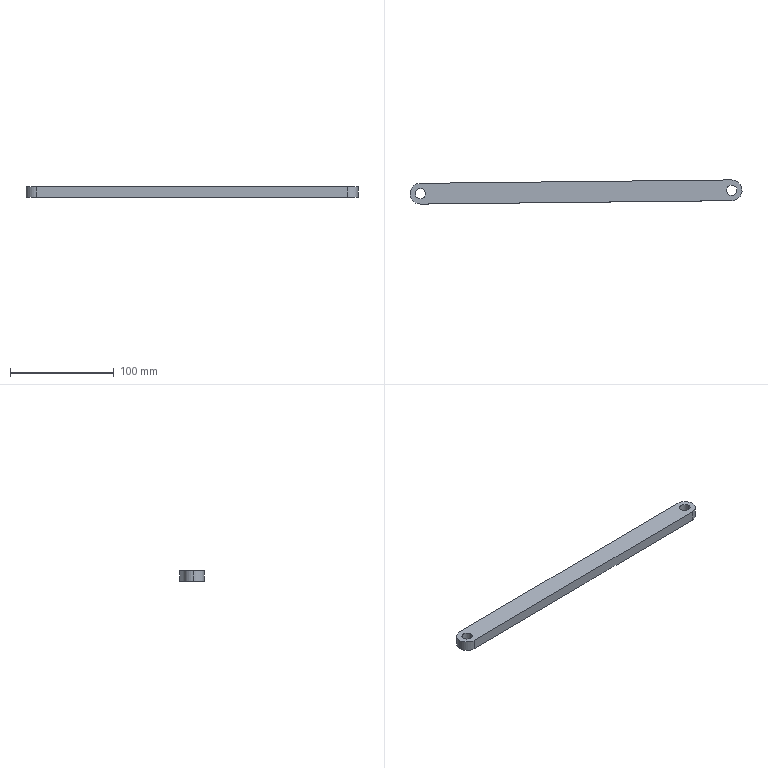Part | SolidWorks | features Extrusion 1 | 1 solid | 11 faces | box 319.982 x 23.296 x 10 mm | volume 61571 mm3 | cylinder 7 | plane 4 | commonest cylinder face diameters 10 x4 20 x3
STEP:
#1=CARTESIAN_POINT('',(-5.,0.,10.));
#2=VERTEX_POINT('',#1);
#3=CARTESIAN_POINT('',(5.,0.,10.));
#4=VERTEX_POINT('',#3);
#5=CARTESIAN_POINT('',(0.,0.,10.));
#6=DIRECTION('',(0.,0.,1.));
#7=DIRECTION('',(1.,0.,0.));
#8=AXIS2_PLACEMENT_3D('',#5,#6,#7);
#9=CIRCLE('',#8,5.);
#10=EDGE_CURVE('',#2,#4,#9,.T.);
#11=ORIENTED_EDGE('',*,*,#10,.T.);
#12=CARTESIAN_POINT('',(5.,0.,0.));
#13=VERTEX_POINT('',#12);
#14=CARTESIAN_POINT('',(5.,0.,10.));
#15=DIRECTION('',(0.,0.,-1.));
#16=VECTOR('',#15,1000.);
#17=LINE('',#14,#16);
#18=EDGE_CURVE('',#4,#13,#17,.T.);
#19=ORIENTED_EDGE('',*,*,#18,.T.);
#20=CARTESIAN_POINT('',(-5.,0.,0.));
#21=VERTEX_POINT('',#20);
#22=CARTESIAN_POINT('',(0.,0.,0.));
#23=DIRECTION('',(0.,0.,1.));
#24=DIRECTION('',(1.,0.,0.));
#25=AXIS2_PLACEMENT_3D('',#22,#23,#24);
#26=CIRCLE('',#25,5.);
#27=EDGE_CURVE('',#21,#13,#26,.T.);
#28=ORIENTED_EDGE('',*,*,#27,.F.);
#29=CARTESIAN_POINT('',(-5.,0.,10.));
#30=DIRECTION('',(0.,0.,-1.));
#31=VECTOR('',#30,1000.);
#32=LINE('',#29,#31);
#33=EDGE_CURVE('',#2,#21,#32,.T.);
#34=ORIENTED_EDGE('',*,*,#33,.F.);
#35=EDGE_LOOP('',(#11,#19,#28,#34));
#36=FACE_OUTER_BOUND('',#35,.T.);
#37=CARTESIAN_POINT('',(0.,0.,10.));
#38=DIRECTION('',(0.,0.,-1.));
#39=DIRECTION('',(-1.,0.,0.));
#40=AXIS2_PLACEMENT_3D('',#37,#38,#39);
#41=CYLINDRICAL_SURFACE('',#40,5.);
#42=ADVANCED_FACE('',(#36),#41,.F.);
#43=CARTESIAN_POINT('',(294.982,3.296,10.));
#44=VERTEX_POINT('',#43);
#45=CARTESIAN_POINT('',(304.982,3.296,10.));
#46=VERTEX_POINT('',#45);
#47=CARTESIAN_POINT('',(299.982,3.296,10.));
#48=DIRECTION('',(0.,0.,1.));
#49=DIRECTION('',(1.,0.,0.));
#50=AXIS2_PLACEMENT_3D('',#47,#48,#49);
#51=CIRCLE('',#50,5.);
#52=EDGE_CURVE('',#44,#46,#51,.T.);
#53=ORIENTED_EDGE('',*,*,#52,.T.);
#54=CARTESIAN_POINT('',(304.982,3.296,0.));
#55=VERTEX_POINT('',#54);
#56=CARTESIAN_POINT('',(304.982,3.296,10.));
#57=DIRECTION('',(0.,0.,-1.));
#58=VECTOR('',#57,1000.);
#59=LINE('',#56,#58);
#60=EDGE_CURVE('',#46,#55,#59,.T.);
#61=ORIENTED_EDGE('',*,*,#60,.T.);
#62=CARTESIAN_POINT('',(294.982,3.296,0.));
#63=VERTEX_POINT('',#62);
#64=CARTESIAN_POINT('',(299.982,3.296,0.));
#65=DIRECTION('',(0.,0.,1.));
#66=DIRECTION('',(1.,0.,0.));
#67=AXIS2_PLACEMENT_3D('',#64,#65,#66);
#68=CIRCLE('',#67,5.);
#69=EDGE_CURVE('',#63,#55,#68,.T.);
#70=ORIENTED_EDGE('',*,*,#69,.F.);
#71=CARTESIAN_POINT('',(294.982,3.296,10.));
#72=DIRECTION('',(0.,0.,-1.));
#73=VECTOR('',#72,1000.);
#74=LINE('',#71,#73);
#75=EDGE_CURVE('',#44,#63,#74,.T.);
#76=ORIENTED_EDGE('',*,*,#75,.F.);
#77=EDGE_LOOP('',(#53,#61,#70,#76));
#78=FACE_OUTER_BOUND('',#77,.T.);
#79=CARTESIAN_POINT('',(299.982,3.296,10.));
#80=DIRECTION('',(0.,0.,-1.));
#81=DIRECTION('',(-1.,0.,0.));
#82=AXIS2_PLACEMENT_3D('',#79,#80,#81);
#83=CYLINDRICAL_SURFACE('',#82,5.);
#84=ADVANCED_FACE('',(#78),#83,.F.);
#85=CARTESIAN_POINT('',(-10.,0.,10.));
#86=VERTEX_POINT('',#85);
#87=CARTESIAN_POINT('',(0.1099,-9.999,10.));
#88=VERTEX_POINT('',#87);
#89=CARTESIAN_POINT('',(0.,0.,10.));
#90=DIRECTION('',(0.,0.,1.));
#91=DIRECTION('',(1.,0.,0.));
#92=AXIS2_PLACEMENT_3D('',#89,#90,#91);
#93=CIRCLE('',#92,10.);
#94=EDGE_CURVE('',#86,#88,#93,.T.);
#95=ORIENTED_EDGE('',*,*,#94,.F.);
#96=CARTESIAN_POINT('',(-10.,0.,0.));
#97=VERTEX_POINT('',#96);
#98=CARTESIAN_POINT('',(-10.,0.,10.));
#99=DIRECTION('',(0.,0.,-1.));
#100=VECTOR('',#99,1000.);
#101=LINE('',#98,#100);
#102=EDGE_CURVE('',#86,#97,#101,.T.);
#103=ORIENTED_EDGE('',*,*,#102,.T.);
#104=CARTESIAN_POINT('',(0.1099,-9.999,0.));
#105=VERTEX_POINT('',#104);
#106=CARTESIAN_POINT('',(0.,0.,0.));
#107=DIRECTION('',(0.,0.,1.));
#108=DIRECTION('',(1.,0.,0.));
#109=AXIS2_PLACEMENT_3D('',#106,#107,#108);
#110=CIRCLE('',#109,10.);
#111=EDGE_CURVE('',#97,#105,#110,.T.);
#112=ORIENTED_EDGE('',*,*,#111,.T.);
#113=CARTESIAN_POINT('',(0.1099,-9.999,10.));
#114=DIRECTION('',(0.,0.,-1.));
#115=VECTOR('',#114,1000.);
#116=LINE('',#113,#115);
#117=EDGE_CURVE('',#88,#105,#116,.T.);
#118=ORIENTED_EDGE('',*,*,#117,.F.);
#119=EDGE_LOOP('',(#95,#103,#112,#118));
#120=FACE_OUTER_BOUND('',#119,.T.);
#121=CARTESIAN_POINT('',(0.,0.,10.));
#122=DIRECTION('',(0.,0.,-1.));
#123=DIRECTION('',(-1.,0.,0.));
#124=AXIS2_PLACEMENT_3D('',#121,#122,#123);
#125=CYLINDRICAL_SURFACE('',#124,10.);
#126=ADVANCED_FACE('',(#120),#125,.T.);
#127=ORIENTED_EDGE('',*,*,#52,.F.);
#128=CARTESIAN_POINT('',(299.982,3.296,10.));
#129=DIRECTION('',(0.,0.,1.));
#130=DIRECTION('',(1.,0.,0.));
#131=AXIS2_PLACEMENT_3D('',#128,#129,#130);
#132=CIRCLE('',#131,5.);
#133=EDGE_CURVE('',#46,#44,#132,.T.);
#134=ORIENTED_EDGE('',*,*,#133,.F.);
#135=EDGE_LOOP('',(#127,#134));
#136=FACE_BOUND('',#135,.T.);
#137=CARTESIAN_POINT('',(-0.1099,9.999,10.));
#138=VERTEX_POINT('',#137);
#139=CARTESIAN_POINT('',(0.,0.,10.));
#140=DIRECTION('',(0.,0.,1.));
#141=DIRECTION('',(1.,0.,0.));
#142=AXIS2_PLACEMENT_3D('',#139,#140,#141);
#143=CIRCLE('',#142,10.);
#144=EDGE_CURVE('',#138,#86,#143,.T.);
#145=ORIENTED_EDGE('',*,*,#144,.T.);
#146=ORIENTED_EDGE('',*,*,#94,.T.);
#147=CARTESIAN_POINT('',(300.092,-6.704,10.));
#148=VERTEX_POINT('',#147);
#149=CARTESIAN_POINT('',(0.1099,-9.999,10.));
#150=DIRECTION('',(0.9999,0.01099,0.));
#151=VECTOR('',#150,1000.);
#152=LINE('',#149,#151);
#153=EDGE_CURVE('',#88,#148,#152,.T.);
#154=ORIENTED_EDGE('',*,*,#153,.T.);
#155=CARTESIAN_POINT('',(299.872,13.295,10.));
#156=VERTEX_POINT('',#155);
#157=CARTESIAN_POINT('',(299.982,3.296,10.));
#158=DIRECTION('',(0.,0.,1.));
#159=DIRECTION('',(1.,0.,0.));
#160=AXIS2_PLACEMENT_3D('',#157,#158,#159);
#161=CIRCLE('',#160,10.);
#162=EDGE_CURVE('',#148,#156,#161,.T.);
#163=ORIENTED_EDGE('',*,*,#162,.T.);
#164=CARTESIAN_POINT('',(-0.1099,9.999,10.));
#165=DIRECTION('',(-0.9999,-0.01099,0.));
#166=VECTOR('',#165,1000.);
#167=LINE('',#164,#166);
#168=EDGE_CURVE('',#156,#138,#167,.T.);
#169=ORIENTED_EDGE('',*,*,#168,.T.);
#170=EDGE_LOOP('',(#145,#146,#154,#163,#169));
#171=FACE_OUTER_BOUND('',#170,.T.);
#172=ORIENTED_EDGE('',*,*,#10,.F.);
#173=CARTESIAN_POINT('',(0.,0.,10.));
#174=DIRECTION('',(0.,0.,1.));
#175=DIRECTION('',(1.,0.,0.));
#176=AXIS2_PLACEMENT_3D('',#173,#174,#175);
#177=CIRCLE('',#176,5.);
#178=EDGE_CURVE('',#4,#2,#177,.T.);
#179=ORIENTED_EDGE('',*,*,#178,.F.);
#180=EDGE_LOOP('',(#172,#179));
#181=FACE_BOUND('',#180,.T.);
#182=CARTESIAN_POINT('',(0.,0.,10.));
#183=DIRECTION('',(0.,0.,1.));
#184=DIRECTION('',(1.,0.,0.));
#185=AXIS2_PLACEMENT_3D('',#182,#183,#184);
#186=PLANE('',#185);
#187=ADVANCED_FACE('',(#136,#171,#181),#186,.T.);
#188=ORIENTED_EDGE('',*,*,#69,.T.);
#189=CARTESIAN_POINT('',(299.982,3.296,0.));
#190=DIRECTION('',(0.,0.,1.));
#191=DIRECTION('',(1.,0.,0.));
#192=AXIS2_PLACEMENT_3D('',#189,#190,#191);
#193=CIRCLE('',#192,5.);
#194=EDGE_CURVE('',#55,#63,#193,.T.);
#195=ORIENTED_EDGE('',*,*,#194,.T.);
#196=EDGE_LOOP('',(#188,#195));
#197=FACE_BOUND('',#196,.T.);
#198=CARTESIAN_POINT('',(-0.1099,9.999,0.));
#199=VERTEX_POINT('',#198);
#200=CARTESIAN_POINT('',(0.,0.,0.));
#201=DIRECTION('',(0.,0.,1.));
#202=DIRECTION('',(1.,0.,0.));
#203=AXIS2_PLACEMENT_3D('',#200,#201,#202);
#204=CIRCLE('',#203,10.);
#205=EDGE_CURVE('',#199,#97,#204,.T.);
#206=ORIENTED_EDGE('',*,*,#205,.F.);
#207=CARTESIAN_POINT('',(299.872,13.295,0.));
#208=VERTEX_POINT('',#207);
#209=CARTESIAN_POINT('',(-0.1099,9.999,0.));
#210=DIRECTION('',(-0.9999,-0.01099,0.));
#211=VECTOR('',#210,1000.);
#212=LINE('',#209,#211);
#213=EDGE_CURVE('',#208,#199,#212,.T.);
#214=ORIENTED_EDGE('',*,*,#213,.F.);
#215=CARTESIAN_POINT('',(300.092,-6.704,0.));
#216=VERTEX_POINT('',#215);
#217=CARTESIAN_POINT('',(299.982,3.296,0.));
#218=DIRECTION('',(0.,0.,1.));
#219=DIRECTION('',(1.,0.,0.));
#220=AXIS2_PLACEMENT_3D('',#217,#218,#219);
#221=CIRCLE('',#220,10.);
#222=EDGE_CURVE('',#216,#208,#221,.T.);
#223=ORIENTED_EDGE('',*,*,#222,.F.);
#224=CARTESIAN_POINT('',(0.1099,-9.999,0.));
#225=DIRECTION('',(0.9999,0.01099,0.));
#226=VECTOR('',#225,1000.);
#227=LINE('',#224,#226);
#228=EDGE_CURVE('',#105,#216,#227,.T.);
#229=ORIENTED_EDGE('',*,*,#228,.F.);
#230=ORIENTED_EDGE('',*,*,#111,.F.);
#231=EDGE_LOOP('',(#206,#214,#223,#229,#230));
#232=FACE_OUTER_BOUND('',#231,.T.);
#233=ORIENTED_EDGE('',*,*,#27,.T.);
#234=CARTESIAN_POINT('',(0.,0.,0.));
#235=DIRECTION('',(0.,0.,1.));
#236=DIRECTION('',(1.,0.,0.));
#237=AXIS2_PLACEMENT_3D('',#234,#235,#236);
#238=CIRCLE('',#237,5.);
#239=EDGE_CURVE('',#13,#21,#238,.T.);
#240=ORIENTED_EDGE('',*,*,#239,.T.);
#241=EDGE_LOOP('',(#233,#240));
#242=FACE_BOUND('',#241,.T.);
#243=CARTESIAN_POINT('',(0.,0.,0.));
#244=DIRECTION('',(0.,0.,1.));
#245=DIRECTION('',(1.,0.,0.));
#246=AXIS2_PLACEMENT_3D('',#243,#244,#245);
#247=PLANE('',#246);
#248=ADVANCED_FACE('',(#197,#232,#242),#247,.F.);
#249=ORIENTED_EDGE('',*,*,#102,.F.);
#250=ORIENTED_EDGE('',*,*,#144,.F.);
#251=CARTESIAN_POINT('',(-0.1099,9.999,10.));
#252=DIRECTION('',(0.,0.,-1.));
#253=VECTOR('',#252,1000.);
#254=LINE('',#251,#253);
#255=EDGE_CURVE('',#138,#199,#254,.T.);
#256=ORIENTED_EDGE('',*,*,#255,.T.);
#257=ORIENTED_EDGE('',*,*,#205,.T.);
#258=EDGE_LOOP('',(#249,#250,#256,#257));
#259=FACE_OUTER_BOUND('',#258,.T.);
#260=CARTESIAN_POINT('',(0.,0.,10.));
#261=DIRECTION('',(0.,0.,-1.));
#262=DIRECTION('',(-1.,0.,0.));
#263=AXIS2_PLACEMENT_3D('',#260,#261,#262);
#264=CYLINDRICAL_SURFACE('',#263,10.);
#265=ADVANCED_FACE('',(#259),#264,.T.);
#266=ORIENTED_EDGE('',*,*,#228,.T.);
#267=CARTESIAN_POINT('',(300.092,-6.704,10.));
#268=DIRECTION('',(0.,0.,-1.));
#269=VECTOR('',#268,1000.);
#270=LINE('',#267,#269);
#271=EDGE_CURVE('',#148,#216,#270,.T.);
#272=ORIENTED_EDGE('',*,*,#271,.F.);
#273=ORIENTED_EDGE('',*,*,#153,.F.);
#274=ORIENTED_EDGE('',*,*,#117,.T.);
#275=EDGE_LOOP('',(#266,#272,#273,#274));
#276=FACE_OUTER_BOUND('',#275,.T.);
#277=CARTESIAN_POINT('',(0.1099,-9.999,10.));
#278=DIRECTION('',(-0.01099,0.9999,0.));
#279=DIRECTION('',(-0.9999,-0.01099,0.));
#280=AXIS2_PLACEMENT_3D('',#277,#278,#279);
#281=PLANE('',#280);
#282=ADVANCED_FACE('',(#276),#281,.F.);
#283=ORIENTED_EDGE('',*,*,#222,.T.);
#284=CARTESIAN_POINT('',(299.872,13.295,10.));
#285=DIRECTION('',(0.,0.,-1.));
#286=VECTOR('',#285,1000.);
#287=LINE('',#284,#286);
#288=EDGE_CURVE('',#156,#208,#287,.T.);
#289=ORIENTED_EDGE('',*,*,#288,.F.);
#290=ORIENTED_EDGE('',*,*,#162,.F.);
#291=ORIENTED_EDGE('',*,*,#271,.T.);
#292=EDGE_LOOP('',(#283,#289,#290,#291));
#293=FACE_OUTER_BOUND('',#292,.T.);
#294=CARTESIAN_POINT('',(299.982,3.296,10.));
#295=DIRECTION('',(0.,0.,-1.));
#296=DIRECTION('',(-1.,0.,0.));
#297=AXIS2_PLACEMENT_3D('',#294,#295,#296);
#298=CYLINDRICAL_SURFACE('',#297,10.);
#299=ADVANCED_FACE('',(#293),#298,.T.);
#300=ORIENTED_EDGE('',*,*,#213,.T.);
#301=ORIENTED_EDGE('',*,*,#255,.F.);
#302=ORIENTED_EDGE('',*,*,#168,.F.);
#303=ORIENTED_EDGE('',*,*,#288,.T.);
#304=EDGE_LOOP('',(#300,#301,#302,#303));
#305=FACE_OUTER_BOUND('',#304,.T.);
#306=CARTESIAN_POINT('',(-0.1099,9.999,10.));
#307=DIRECTION('',(0.01099,-0.9999,0.));
#308=DIRECTION('',(0.9999,0.01099,0.));
#309=AXIS2_PLACEMENT_3D('',#306,#307,#308);
#310=PLANE('',#309);
#311=ADVANCED_FACE('',(#305),#310,.F.);
#312=ORIENTED_EDGE('',*,*,#60,.F.);
#313=ORIENTED_EDGE('',*,*,#133,.T.);
#314=ORIENTED_EDGE('',*,*,#75,.T.);
#315=ORIENTED_EDGE('',*,*,#194,.F.);
#316=EDGE_LOOP('',(#312,#313,#314,#315));
#317=FACE_OUTER_BOUND('',#316,.T.);
#318=CARTESIAN_POINT('',(299.982,3.296,10.));
#319=DIRECTION('',(0.,0.,-1.));
#320=DIRECTION('',(-1.,0.,0.));
#321=AXIS2_PLACEMENT_3D('',#318,#319,#320);
#322=CYLINDRICAL_SURFACE('',#321,5.);
#323=ADVANCED_FACE('',(#317),#322,.F.);
#324=ORIENTED_EDGE('',*,*,#18,.F.);
#325=ORIENTED_EDGE('',*,*,#178,.T.);
#326=ORIENTED_EDGE('',*,*,#33,.T.);
#327=ORIENTED_EDGE('',*,*,#239,.F.);
#328=EDGE_LOOP('',(#324,#325,#326,#327));
#329=FACE_OUTER_BOUND('',#328,.T.);
#330=CARTESIAN_POINT('',(0.,0.,10.));
#331=DIRECTION('',(0.,0.,-1.));
#332=DIRECTION('',(-1.,0.,0.));
#333=AXIS2_PLACEMENT_3D('',#330,#331,#332);
#334=CYLINDRICAL_SURFACE('',#333,5.);
#335=ADVANCED_FACE('',(#329),#334,.F.);
#336=CLOSED_SHELL('',(#42,#84,#126,#187,#248,#265,#282,#299,#311,#323,#335));
#337=MANIFOLD_SOLID_BREP('',#336);
#338=CARTESIAN_POINT('',(0.,0.,0.));
#339=DIRECTION('',(0.,0.,1.));
#340=DIRECTION('',(1.,0.,0.));
#341=AXIS2_PLACEMENT_3D('',#338,#339,#340);
#342=(LENGTH_UNIT()NAMED_UNIT(*)SI_UNIT(.MILLI.,.METRE.));
#343=UNCERTAINTY_MEASURE_WITH_UNIT(LENGTH_MEASURE(0.00001),#342,'','');
#344=(NAMED_UNIT(*)PLANE_ANGLE_UNIT()SI_UNIT($,.RADIAN.));
#345=(NAMED_UNIT(*)SI_UNIT($,.STERADIAN.)SOLID_ANGLE_UNIT());
#346=(GEOMETRIC_REPRESENTATION_CONTEXT(3)GLOBAL_UNCERTAINTY_ASSIGNED_CONTEXT((#343))GLOBAL_UNIT_ASSIGNED_CONTEXT((#342,#344,#345))REPRESENTATION_CONTEXT('',''));
#347=ADVANCED_BREP_SHAPE_REPRESENTATION('',(#337,#341),#346);